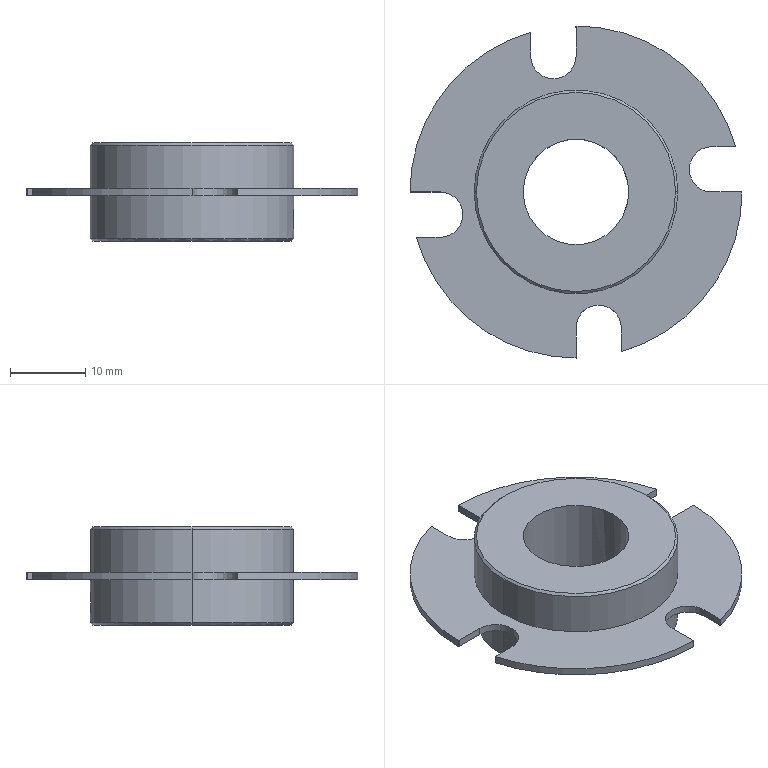Part | NX | 1 solid | 44 faces | box 44 x 44 x 13 mm | volume 6172 mm3 | cylinder 24 | plane 12 | spline 4 | cone 4 | commonest cylinder face diameters 6 x9 44 x5 2.5 x4 27 x4 14 x2